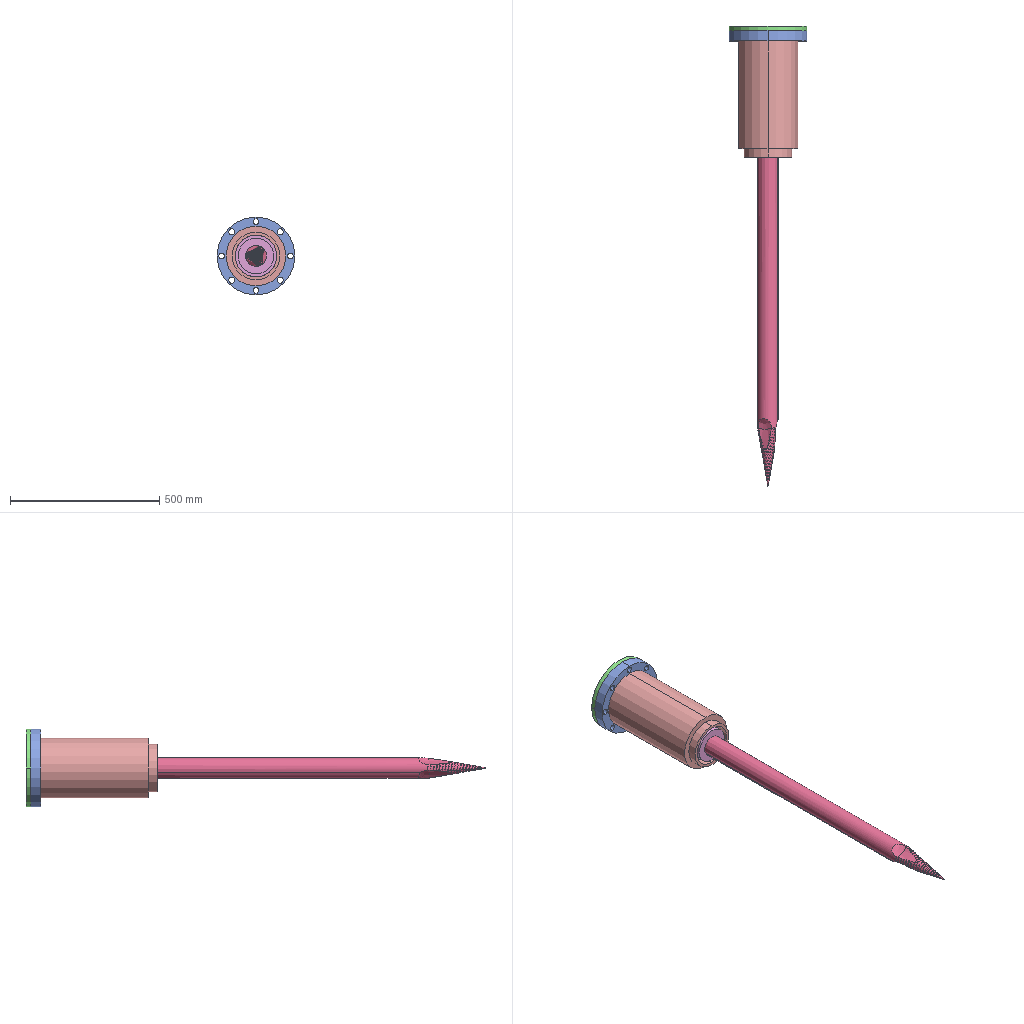Assembly | SolidWorks | 8 different items | 10 placed | box 260 x 1540 x 260 mm
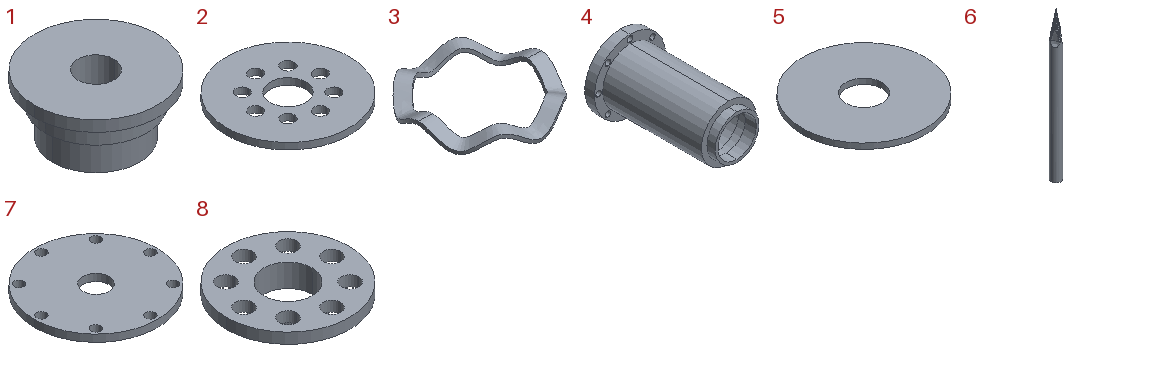Parts list (item | quantity | size | volume | features):
1 | x1 | 170 x 170 x 81 mm | 1034055 mm3 | features ICE 2, Cut 1, Extrusion 1
2 | x1 | 190 x 190 x 10 mm | 234638 mm3 | features CirPattern 1, Cut 1, Extrusion 1
3 | x2 | 180 x 180.809 x 25.967 mm | 56026 mm3 | features 3DProfileFeature 2, 3DSplineCurve 1, Extrusion 1, Sweep 1
4 | x1 | 260 x 425 x 260 mm | 2163536 mm3 | features Cut 3, ICE 2, CirPattern 1, Extrusion 1, Shell 1
5 | x2 | 170 x 170 x 7.5 mm | 155509 mm3 | features Cut 1, Extrusion 1
6 | x1 | 70 x 70 x 1100 mm | 2879786 mm3 | features Chamfer 2, Fillet 2, Cut 1, Extrusion 1, Helix 1, ICE 1, SweepCut 1
7 | x1 | 260 x 260 x 15 mm | 723057 mm3 | features CirPattern 1, Cut 1, Extrusion 1
8 | x1 | 140 x 140 x 26 mm | 142154 mm3 | features CirPattern 1, Cut 1, Extrusion 1, ICE 1
Mates (type | each side: item.copy, entity, surface, feature):
Concentric | 4.1 face cylinder Shell1 | 3.1 select_type:24
Coincident | 4.1 face plane Shell1 | 3.1 select_type:24
Coincident | 3.1 plane | 1.1 face plane Boss-Extrude2
Concentric | 4.1 face cylinder Boss-Extrude1 | 1.1 face cylinder Boss-Extrude2
Concentric | 1.1 face cylinder Boss-Extrude2 | 5.1 face cylinder Boss-Extrude1
Coincident | 1.1 face plane Boss-Extrude2 | 5.1 face plane Boss-Extrude1
Coincident | 5.1 face plane Boss-Extrude1 | assembly face
Concentric | 4.1 face cylinder Boss-Extrude1 | assembly face | 24 times
Coincident | assembly face | assembly face | 19 times
Concentric | 4.1 face cylinder Boss-Extrude1 | 5.2 face cylinder Boss-Extrude1
Coincident | assembly face | 5.2 face plane Boss-Extrude1
Width | assembly face | assembly face | assembly face | assembly face
Concentric | assembly face | assembly face | 2 times
Coincident | assembly face | assembly edge | 6 times
Concentric | 4.1 face cylinder Boss-Extrude3 | assembly face
Coincident | 5.2 face plane Boss-Extrude1 | 2.1 face plane Boss-Extrude1
Concentric | 5.2 edge | 2.1 edge
Coincident | 2.1 face plane Boss-Extrude1 | 8.1 face plane Boss-Extrude1
Concentric | 2.1 face cylinder Cut-Extrude1 | 8.1 face cylinder CirPattern1
Coincident | 2.1 face plane Boss-Extrude1 | 3.2 plane
Concentric | 8.1 edge | 3.2 select_type:24
InPlace | 5.2 face plane Boss-Extrude1 | assembly plane
InPlace | 4.1 face plane Boss-Extrude3 | 7.1 plane
InPlace | 1.1 face plane Boss-Extrude3 | 6.1 plane